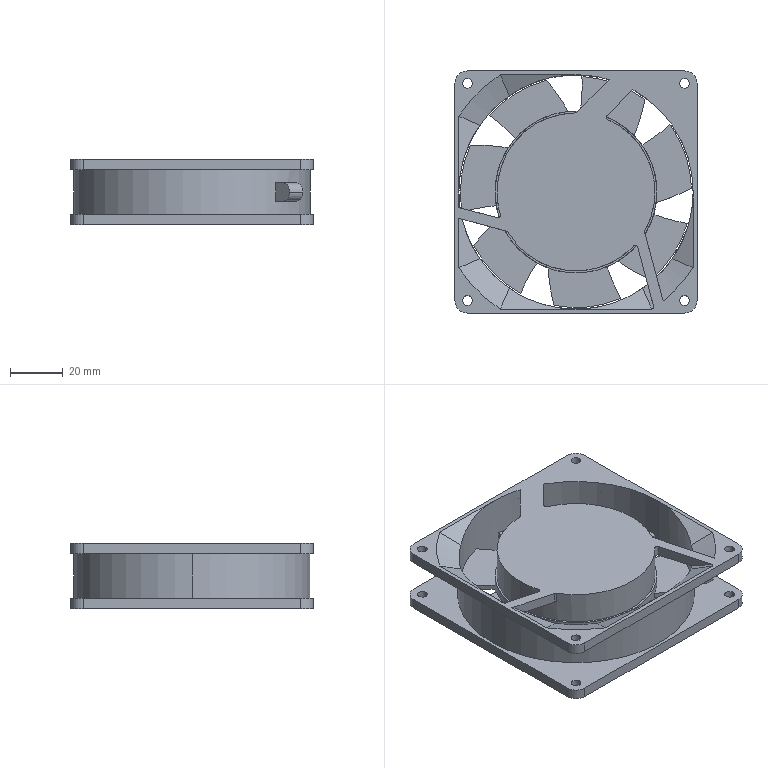Part | STEP file | 1_2_1-- | 1 solid | 136 faces | box 92 x 92 x 25 mm | volume 97841 mm3 | cylinder 66 | plane 62 | cone 8 | commonest cylinder face diameters 3.7 x16 9.5 x8 87.8 x8 2 x7 149.02 x7 153.9 x7